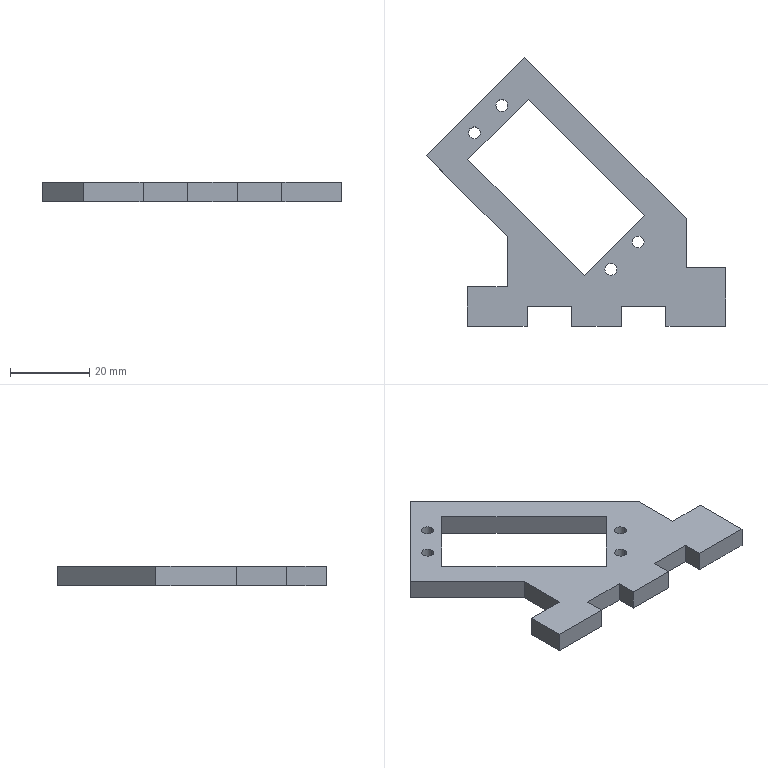Part | SolidWorks | features Extrusion 1 | 1 solid | 32 faces | box 75.329 x 67.7 x 5 mm | volume 9212 mm3 | plane 24 | cylinder 8 | commonest cylinder face diameters 3 x8
STEP:
#1=CARTESIAN_POINT('',(9.961,-20.341,5.));
#2=VERTEX_POINT('',#1);
#3=CARTESIAN_POINT('',(6.961,-20.341,5.));
#4=VERTEX_POINT('',#3);
#5=CARTESIAN_POINT('',(8.461,-20.341,5.));
#6=DIRECTION('',(0.,0.,-1.));
#7=DIRECTION('',(1.,0.,0.));
#8=AXIS2_PLACEMENT_3D('',#5,#6,#7);
#9=CIRCLE('',#8,1.5);
#10=EDGE_CURVE('',#2,#4,#9,.T.);
#11=ORIENTED_EDGE('',*,*,#10,.F.);
#12=CARTESIAN_POINT('',(9.961,-20.341,0.));
#13=VERTEX_POINT('',#12);
#14=CARTESIAN_POINT('',(9.961,-20.341,5.));
#15=DIRECTION('',(0.,0.,-1.));
#16=VECTOR('',#15,1000.);
#17=LINE('',#14,#16);
#18=EDGE_CURVE('',#2,#13,#17,.T.);
#19=ORIENTED_EDGE('',*,*,#18,.T.);
#20=CARTESIAN_POINT('',(6.961,-20.341,0.));
#21=VERTEX_POINT('',#20);
#22=CARTESIAN_POINT('',(8.461,-20.341,0.));
#23=DIRECTION('',(0.,0.,-1.));
#24=DIRECTION('',(1.,0.,0.));
#25=AXIS2_PLACEMENT_3D('',#22,#23,#24);
#26=CIRCLE('',#25,1.5);
#27=EDGE_CURVE('',#13,#21,#26,.T.);
#28=ORIENTED_EDGE('',*,*,#27,.T.);
#29=CARTESIAN_POINT('',(6.961,-20.341,5.));
#30=DIRECTION('',(0.,0.,-1.));
#31=VECTOR('',#30,1000.);
#32=LINE('',#29,#31);
#33=EDGE_CURVE('',#4,#21,#32,.T.);
#34=ORIENTED_EDGE('',*,*,#33,.F.);
#35=EDGE_LOOP('',(#11,#19,#28,#34));
#36=FACE_OUTER_BOUND('',#35,.T.);
#37=CARTESIAN_POINT('',(8.461,-20.341,5.));
#38=DIRECTION('',(0.,0.,-1.));
#39=DIRECTION('',(-1.,0.,0.));
#40=AXIS2_PLACEMENT_3D('',#37,#38,#39);
#41=CYLINDRICAL_SURFACE('',#40,1.5);
#42=ADVANCED_FACE('',(#36),#41,.F.);
#43=CARTESIAN_POINT('',(-20.51,20.918,5.));
#44=VERTEX_POINT('',#43);
#45=CARTESIAN_POINT('',(-17.51,20.918,5.));
#46=VERTEX_POINT('',#45);
#47=CARTESIAN_POINT('',(-19.01,20.918,5.));
#48=DIRECTION('',(0.,0.,1.));
#49=DIRECTION('',(1.,0.,0.));
#50=AXIS2_PLACEMENT_3D('',#47,#48,#49);
#51=CIRCLE('',#50,1.5);
#52=EDGE_CURVE('',#44,#46,#51,.T.);
#53=ORIENTED_EDGE('',*,*,#52,.T.);
#54=CARTESIAN_POINT('',(-17.51,20.918,0.));
#55=VERTEX_POINT('',#54);
#56=CARTESIAN_POINT('',(-17.51,20.918,5.));
#57=DIRECTION('',(0.,0.,-1.));
#58=VECTOR('',#57,1000.);
#59=LINE('',#56,#58);
#60=EDGE_CURVE('',#46,#55,#59,.T.);
#61=ORIENTED_EDGE('',*,*,#60,.T.);
#62=CARTESIAN_POINT('',(-20.51,20.918,0.));
#63=VERTEX_POINT('',#62);
#64=CARTESIAN_POINT('',(-19.01,20.918,0.));
#65=DIRECTION('',(0.,0.,1.));
#66=DIRECTION('',(1.,0.,0.));
#67=AXIS2_PLACEMENT_3D('',#64,#65,#66);
#68=CIRCLE('',#67,1.5);
#69=EDGE_CURVE('',#63,#55,#68,.T.);
#70=ORIENTED_EDGE('',*,*,#69,.F.);
#71=CARTESIAN_POINT('',(-20.51,20.918,5.));
#72=DIRECTION('',(0.,0.,-1.));
#73=VECTOR('',#72,1000.);
#74=LINE('',#71,#73);
#75=EDGE_CURVE('',#44,#63,#74,.T.);
#76=ORIENTED_EDGE('',*,*,#75,.F.);
#77=EDGE_LOOP('',(#53,#61,#70,#76));
#78=FACE_OUTER_BOUND('',#77,.T.);
#79=CARTESIAN_POINT('',(-19.01,20.918,5.));
#80=DIRECTION('',(0.,0.,-1.));
#81=DIRECTION('',(-1.,0.,0.));
#82=AXIS2_PLACEMENT_3D('',#79,#80,#81);
#83=CYLINDRICAL_SURFACE('',#82,1.5);
#84=ADVANCED_FACE('',(#78),#83,.F.);
#85=CARTESIAN_POINT('',(16.856,-13.447,5.));
#86=VERTEX_POINT('',#85);
#87=CARTESIAN_POINT('',(13.856,-13.447,5.));
#88=VERTEX_POINT('',#87);
#89=CARTESIAN_POINT('',(15.356,-13.447,5.));
#90=DIRECTION('',(0.,0.,-1.));
#91=DIRECTION('',(1.,0.,0.));
#92=AXIS2_PLACEMENT_3D('',#89,#90,#91);
#93=CIRCLE('',#92,1.5);
#94=EDGE_CURVE('',#86,#88,#93,.T.);
#95=ORIENTED_EDGE('',*,*,#94,.F.);
#96=CARTESIAN_POINT('',(16.856,-13.447,0.));
#97=VERTEX_POINT('',#96);
#98=CARTESIAN_POINT('',(16.856,-13.447,5.));
#99=DIRECTION('',(0.,0.,-1.));
#100=VECTOR('',#99,1000.);
#101=LINE('',#98,#100);
#102=EDGE_CURVE('',#86,#97,#101,.T.);
#103=ORIENTED_EDGE('',*,*,#102,.T.);
#104=CARTESIAN_POINT('',(13.856,-13.447,0.));
#105=VERTEX_POINT('',#104);
#106=CARTESIAN_POINT('',(15.356,-13.447,0.));
#107=DIRECTION('',(0.,0.,-1.));
#108=DIRECTION('',(1.,0.,0.));
#109=AXIS2_PLACEMENT_3D('',#106,#107,#108);
#110=CIRCLE('',#109,1.5);
#111=EDGE_CURVE('',#97,#105,#110,.T.);
#112=ORIENTED_EDGE('',*,*,#111,.T.);
#113=CARTESIAN_POINT('',(13.856,-13.447,5.));
#114=DIRECTION('',(0.,0.,-1.));
#115=VECTOR('',#114,1000.);
#116=LINE('',#113,#115);
#117=EDGE_CURVE('',#88,#105,#116,.T.);
#118=ORIENTED_EDGE('',*,*,#117,.F.);
#119=EDGE_LOOP('',(#95,#103,#112,#118));
#120=FACE_OUTER_BOUND('',#119,.T.);
#121=CARTESIAN_POINT('',(15.356,-13.447,5.));
#122=DIRECTION('',(0.,0.,-1.));
#123=DIRECTION('',(-1.,0.,0.));
#124=AXIS2_PLACEMENT_3D('',#121,#122,#123);
#125=CYLINDRICAL_SURFACE('',#124,1.5);
#126=ADVANCED_FACE('',(#120),#125,.F.);
#127=CARTESIAN_POINT('',(-27.404,14.024,5.));
#128=VERTEX_POINT('',#127);
#129=CARTESIAN_POINT('',(-24.404,14.024,5.));
#130=VERTEX_POINT('',#129);
#131=CARTESIAN_POINT('',(-25.904,14.024,5.));
#132=DIRECTION('',(0.,0.,1.));
#133=DIRECTION('',(1.,0.,0.));
#134=AXIS2_PLACEMENT_3D('',#131,#132,#133);
#135=CIRCLE('',#134,1.5);
#136=EDGE_CURVE('',#128,#130,#135,.T.);
#137=ORIENTED_EDGE('',*,*,#136,.T.);
#138=CARTESIAN_POINT('',(-24.404,14.024,0.));
#139=VERTEX_POINT('',#138);
#140=CARTESIAN_POINT('',(-24.404,14.024,5.));
#141=DIRECTION('',(0.,0.,-1.));
#142=VECTOR('',#141,1000.);
#143=LINE('',#140,#142);
#144=EDGE_CURVE('',#130,#139,#143,.T.);
#145=ORIENTED_EDGE('',*,*,#144,.T.);
#146=CARTESIAN_POINT('',(-27.404,14.024,0.));
#147=VERTEX_POINT('',#146);
#148=CARTESIAN_POINT('',(-25.904,14.024,0.));
#149=DIRECTION('',(0.,0.,1.));
#150=DIRECTION('',(1.,0.,0.));
#151=AXIS2_PLACEMENT_3D('',#148,#149,#150);
#152=CIRCLE('',#151,1.5);
#153=EDGE_CURVE('',#147,#139,#152,.T.);
#154=ORIENTED_EDGE('',*,*,#153,.F.);
#155=CARTESIAN_POINT('',(-27.404,14.024,5.));
#156=DIRECTION('',(0.,0.,-1.));
#157=VECTOR('',#156,1000.);
#158=LINE('',#155,#157);
#159=EDGE_CURVE('',#128,#147,#158,.T.);
#160=ORIENTED_EDGE('',*,*,#159,.F.);
#161=EDGE_LOOP('',(#137,#145,#154,#160));
#162=FACE_OUTER_BOUND('',#161,.T.);
#163=CARTESIAN_POINT('',(-25.904,14.024,5.));
#164=DIRECTION('',(0.,0.,-1.));
#165=DIRECTION('',(-1.,0.,0.));
#166=AXIS2_PLACEMENT_3D('',#163,#164,#165);
#167=CYLINDRICAL_SURFACE('',#166,1.5);
#168=ADVANCED_FACE('',(#162),#167,.F.);
#169=CARTESIAN_POINT('',(-12.649,-29.708,0.));
#170=VERTEX_POINT('',#169);
#171=CARTESIAN_POINT('',(-12.649,-34.708,0.));
#172=VERTEX_POINT('',#171);
#173=CARTESIAN_POINT('',(-12.649,0.,0.));
#174=DIRECTION('',(0.,-1.,0.));
#175=VECTOR('',#174,1000.);
#176=LINE('',#173,#175);
#177=EDGE_CURVE('',#170,#172,#176,.T.);
#178=ORIENTED_EDGE('',*,*,#177,.F.);
#179=CARTESIAN_POINT('',(-12.649,-29.708,5.));
#180=VERTEX_POINT('',#179);
#181=CARTESIAN_POINT('',(-12.649,-29.708,5.));
#182=DIRECTION('',(0.,0.,-1.));
#183=VECTOR('',#182,1000.);
#184=LINE('',#181,#183);
#185=EDGE_CURVE('',#180,#170,#184,.T.);
#186=ORIENTED_EDGE('',*,*,#185,.F.);
#187=CARTESIAN_POINT('',(-12.649,-34.708,5.));
#188=VERTEX_POINT('',#187);
#189=CARTESIAN_POINT('',(-12.649,0.,5.));
#190=DIRECTION('',(0.,-1.,0.));
#191=VECTOR('',#190,1000.);
#192=LINE('',#189,#191);
#193=EDGE_CURVE('',#180,#188,#192,.T.);
#194=ORIENTED_EDGE('',*,*,#193,.T.);
#195=CARTESIAN_POINT('',(-12.649,-34.708,5.));
#196=DIRECTION('',(0.,0.,-1.));
#197=VECTOR('',#196,1000.);
#198=LINE('',#195,#197);
#199=EDGE_CURVE('',#188,#172,#198,.T.);
#200=ORIENTED_EDGE('',*,*,#199,.T.);
#201=EDGE_LOOP('',(#178,#186,#194,#200));
#202=FACE_OUTER_BOUND('',#201,.T.);
#203=CARTESIAN_POINT('',(-12.649,0.,5.));
#204=DIRECTION('',(1.,0.,0.));
#205=DIRECTION('',(0.,0.,-1.));
#206=AXIS2_PLACEMENT_3D('',#203,#204,#205);
#207=PLANE('',#206);
#208=ADVANCED_FACE('',(#202),#207,.T.);
#209=CARTESIAN_POINT('',(-1.399,-29.708,0.));
#210=VERTEX_POINT('',#209);
#211=CARTESIAN_POINT('',(0.,-29.708,0.));
#212=DIRECTION('',(-1.,0.,0.));
#213=VECTOR('',#212,1000.);
#214=LINE('',#211,#213);
#215=EDGE_CURVE('',#210,#170,#214,.T.);
#216=ORIENTED_EDGE('',*,*,#215,.F.);
#217=CARTESIAN_POINT('',(-1.399,-29.708,5.));
#218=VERTEX_POINT('',#217);
#219=CARTESIAN_POINT('',(-1.399,-29.708,5.));
#220=DIRECTION('',(0.,0.,-1.));
#221=VECTOR('',#220,1000.);
#222=LINE('',#219,#221);
#223=EDGE_CURVE('',#218,#210,#222,.T.);
#224=ORIENTED_EDGE('',*,*,#223,.F.);
#225=CARTESIAN_POINT('',(0.,-29.708,5.));
#226=DIRECTION('',(-1.,0.,0.));
#227=VECTOR('',#226,1000.);
#228=LINE('',#225,#227);
#229=EDGE_CURVE('',#218,#180,#228,.T.);
#230=ORIENTED_EDGE('',*,*,#229,.T.);
#231=ORIENTED_EDGE('',*,*,#185,.T.);
#232=EDGE_LOOP('',(#216,#224,#230,#231));
#233=FACE_OUTER_BOUND('',#232,.T.);
#234=CARTESIAN_POINT('',(0.,-29.708,5.));
#235=DIRECTION('',(0.,-1.,0.));
#236=DIRECTION('',(0.,0.,-1.));
#237=AXIS2_PLACEMENT_3D('',#234,#235,#236);
#238=PLANE('',#237);
#239=ADVANCED_FACE('',(#233),#238,.T.);
#240=CARTESIAN_POINT('',(-1.399,-34.708,0.));
#241=VERTEX_POINT('',#240);
#242=CARTESIAN_POINT('',(-1.399,0.,0.));
#243=DIRECTION('',(0.,1.,0.));
#244=VECTOR('',#243,1000.);
#245=LINE('',#242,#244);
#246=EDGE_CURVE('',#241,#210,#245,.T.);
#247=ORIENTED_EDGE('',*,*,#246,.F.);
#248=CARTESIAN_POINT('',(-1.399,-34.708,5.));
#249=VERTEX_POINT('',#248);
#250=CARTESIAN_POINT('',(-1.399,-34.708,5.));
#251=DIRECTION('',(0.,0.,-1.));
#252=VECTOR('',#251,1000.);
#253=LINE('',#250,#252);
#254=EDGE_CURVE('',#249,#241,#253,.T.);
#255=ORIENTED_EDGE('',*,*,#254,.F.);
#256=CARTESIAN_POINT('',(-1.399,0.,5.));
#257=DIRECTION('',(0.,1.,0.));
#258=VECTOR('',#257,1000.);
#259=LINE('',#256,#258);
#260=EDGE_CURVE('',#249,#218,#259,.T.);
#261=ORIENTED_EDGE('',*,*,#260,.T.);
#262=ORIENTED_EDGE('',*,*,#223,.T.);
#263=EDGE_LOOP('',(#247,#255,#261,#262));
#264=FACE_OUTER_BOUND('',#263,.T.);
#265=CARTESIAN_POINT('',(-1.399,0.,5.));
#266=DIRECTION('',(-1.,0.,0.));
#267=DIRECTION('',(0.,-1.,0.));
#268=AXIS2_PLACEMENT_3D('',#265,#266,#267);
#269=PLANE('',#268);
#270=ADVANCED_FACE('',(#264),#269,.T.);
#271=CARTESIAN_POINT('',(11.101,-34.708,0.));
#272=VERTEX_POINT('',#271);
#273=CARTESIAN_POINT('',(0.,-34.708,0.));
#274=DIRECTION('',(-1.,0.,0.));
#275=VECTOR('',#274,1000.);
#276=LINE('',#273,#275);
#277=EDGE_CURVE('',#272,#241,#276,.T.);
#278=ORIENTED_EDGE('',*,*,#277,.F.);
#279=CARTESIAN_POINT('',(11.101,-34.708,5.));
#280=VERTEX_POINT('',#279);
#281=CARTESIAN_POINT('',(11.101,-34.708,5.));
#282=DIRECTION('',(0.,0.,-1.));
#283=VECTOR('',#282,1000.);
#284=LINE('',#281,#283);
#285=EDGE_CURVE('',#280,#272,#284,.T.);
#286=ORIENTED_EDGE('',*,*,#285,.F.);
#287=CARTESIAN_POINT('',(0.,-34.708,5.));
#288=DIRECTION('',(-1.,0.,0.));
#289=VECTOR('',#288,1000.);
#290=LINE('',#287,#289);
#291=EDGE_CURVE('',#280,#249,#290,.T.);
#292=ORIENTED_EDGE('',*,*,#291,.T.);
#293=ORIENTED_EDGE('',*,*,#254,.T.);
#294=EDGE_LOOP('',(#278,#286,#292,#293));
#295=FACE_OUTER_BOUND('',#294,.T.);
#296=CARTESIAN_POINT('',(0.,-34.708,5.));
#297=DIRECTION('',(0.,-1.,0.));
#298=DIRECTION('',(1.,0.,0.));
#299=AXIS2_PLACEMENT_3D('',#296,#297,#298);
#300=PLANE('',#299);
#301=ADVANCED_FACE('',(#295),#300,.T.);
#302=CARTESIAN_POINT('',(11.101,-29.708,0.));
#303=VERTEX_POINT('',#302);
#304=CARTESIAN_POINT('',(11.101,0.,0.));
#305=DIRECTION('',(0.,-1.,0.));
#306=VECTOR('',#305,1000.);
#307=LINE('',#304,#306);
#308=EDGE_CURVE('',#303,#272,#307,.T.);
#309=ORIENTED_EDGE('',*,*,#308,.F.);
#310=CARTESIAN_POINT('',(11.101,-29.708,5.));
#311=VERTEX_POINT('',#310);
#312=CARTESIAN_POINT('',(11.101,-29.708,5.));
#313=DIRECTION('',(0.,0.,-1.));
#314=VECTOR('',#313,1000.);
#315=LINE('',#312,#314);
#316=EDGE_CURVE('',#311,#303,#315,.T.);
#317=ORIENTED_EDGE('',*,*,#316,.F.);
#318=CARTESIAN_POINT('',(11.101,0.,5.));
#319=DIRECTION('',(0.,-1.,0.));
#320=VECTOR('',#319,1000.);
#321=LINE('',#318,#320);
#322=EDGE_CURVE('',#311,#280,#321,.T.);
#323=ORIENTED_EDGE('',*,*,#322,.T.);
#324=ORIENTED_EDGE('',*,*,#285,.T.);
#325=EDGE_LOOP('',(#309,#317,#323,#324));
#326=FACE_OUTER_BOUND('',#325,.T.);
#327=CARTESIAN_POINT('',(11.101,0.,5.));
#328=DIRECTION('',(1.,0.,0.));
#329=DIRECTION('',(0.,0.,-1.));
#330=AXIS2_PLACEMENT_3D('',#327,#328,#329);
#331=PLANE('',#330);
#332=ADVANCED_FACE('',(#326),#331,.T.);
#333=CARTESIAN_POINT('',(22.351,-29.708,0.));
#334=VERTEX_POINT('',#333);
#335=CARTESIAN_POINT('',(0.,-29.708,0.));
#336=DIRECTION('',(-1.,0.,0.));
#337=VECTOR('',#336,1000.);
#338=LINE('',#335,#337);
#339=EDGE_CURVE('',#334,#303,#338,.T.);
#340=ORIENTED_EDGE('',*,*,#339,.F.);
#341=CARTESIAN_POINT('',(22.351,-29.708,5.));
#342=VERTEX_POINT('',#341);
#343=CARTESIAN_POINT('',(22.351,-29.708,5.));
#344=DIRECTION('',(0.,0.,-1.));
#345=VECTOR('',#344,1000.);
#346=LINE('',#343,#345);
#347=EDGE_CURVE('',#342,#334,#346,.T.);
#348=ORIENTED_EDGE('',*,*,#347,.F.);
#349=CARTESIAN_POINT('',(0.,-29.708,5.));
#350=DIRECTION('',(-1.,0.,0.));
#351=VECTOR('',#350,1000.);
#352=LINE('',#349,#351);
#353=EDGE_CURVE('',#342,#311,#352,.T.);
#354=ORIENTED_EDGE('',*,*,#353,.T.);
#355=ORIENTED_EDGE('',*,*,#316,.T.);
#356=EDGE_LOOP('',(#340,#348,#354,#355));
#357=FACE_OUTER_BOUND('',#356,.T.);
#358=CARTESIAN_POINT('',(0.,-29.708,5.));
#359=DIRECTION('',(0.,-1.,0.));
#360=DIRECTION('',(0.,0.,-1.));
#361=AXIS2_PLACEMENT_3D('',#358,#359,#360);
#362=PLANE('',#361);
#363=ADVANCED_FACE('',(#357),#362,.T.);
#364=CARTESIAN_POINT('',(22.351,-34.708,0.));
#365=VERTEX_POINT('',#364);
#366=CARTESIAN_POINT('',(22.351,0.,0.));
#367=DIRECTION('',(0.,1.,0.));
#368=VECTOR('',#367,1000.);
#369=LINE('',#366,#368);
#370=EDGE_CURVE('',#365,#334,#369,.T.);
#371=ORIENTED_EDGE('',*,*,#370,.F.);
#372=CARTESIAN_POINT('',(22.351,-34.708,5.));
#373=VERTEX_POINT('',#372);
#374=CARTESIAN_POINT('',(22.351,-34.708,5.));
#375=DIRECTION('',(0.,0.,-1.));
#376=VECTOR('',#375,1000.);
#377=LINE('',#374,#376);
#378=EDGE_CURVE('',#373,#365,#377,.T.);
#379=ORIENTED_EDGE('',*,*,#378,.F.);
#380=CARTESIAN_POINT('',(22.351,0.,5.));
#381=DIRECTION('',(0.,1.,0.));
#382=VECTOR('',#381,1000.);
#383=LINE('',#380,#382);
#384=EDGE_CURVE('',#373,#342,#383,.T.);
#385=ORIENTED_EDGE('',*,*,#384,.T.);
#386=ORIENTED_EDGE('',*,*,#347,.T.);
#387=EDGE_LOOP('',(#371,#379,#385,#386));
#388=FACE_OUTER_BOUND('',#387,.T.);
#389=CARTESIAN_POINT('',(22.351,0.,5.));
#390=DIRECTION('',(-1.,0.,0.));
#391=DIRECTION('',(0.,0.,1.));
#392=AXIS2_PLACEMENT_3D('',#389,#390,#391);
#393=PLANE('',#392);
#394=ADVANCED_FACE('',(#388),#393,.T.);
#395=CARTESIAN_POINT('',(37.351,-34.708,0.));
#396=VERTEX_POINT('',#395);
#397=CARTESIAN_POINT('',(0.,-34.708,0.));
#398=DIRECTION('',(-1.,0.,0.));
#399=VECTOR('',#398,1000.);
#400=LINE('',#397,#399);
#401=EDGE_CURVE('',#396,#365,#400,.T.);
#402=ORIENTED_EDGE('',*,*,#401,.F.);
#403=CARTESIAN_POINT('',(37.351,-34.708,5.));
#404=VERTEX_POINT('',#403);
#405=CARTESIAN_POINT('',(37.351,-34.708,5.));
#406=DIRECTION('',(0.,0.,-1.));
#407=VECTOR('',#406,1000.);
#408=LINE('',#405,#407);
#409=EDGE_CURVE('',#404,#396,#408,.T.);
#410=ORIENTED_EDGE('',*,*,#409,.F.);
#411=CARTESIAN_POINT('',(0.,-34.708,5.));
#412=DIRECTION('',(-1.,0.,0.));
#413=VECTOR('',#412,1000.);
#414=LINE('',#411,#413);
#415=EDGE_CURVE('',#404,#373,#414,.T.);
#416=ORIENTED_EDGE('',*,*,#415,.T.);
#417=ORIENTED_EDGE('',*,*,#378,.T.);
#418=EDGE_LOOP('',(#402,#410,#416,#417));
#419=FACE_OUTER_BOUND('',#418,.T.);
#420=CARTESIAN_POINT('',(0.,-34.708,5.));
#421=DIRECTION('',(0.,-1.,0.));
#422=DIRECTION('',(0.,0.,-1.));
#423=AXIS2_PLACEMENT_3D('',#420,#421,#422);
#424=PLANE('',#423);
#425=ADVANCED_FACE('',(#419),#424,.T.);
#426=CARTESIAN_POINT('',(37.351,-19.908,0.));
#427=VERTEX_POINT('',#426);
#428=CARTESIAN_POINT('',(37.351,0.,0.));
#429=DIRECTION('',(0.,-1.,0.));
#430=VECTOR('',#429,1000.);
#431=LINE('',#428,#430);
#432=EDGE_CURVE('',#427,#396,#431,.T.);
#433=ORIENTED_EDGE('',*,*,#432,.F.);
#434=CARTESIAN_POINT('',(37.351,-19.908,5.));
#435=VERTEX_POINT('',#434);
#436=CARTESIAN_POINT('',(37.351,-19.908,5.));
#437=DIRECTION('',(0.,0.,-1.));
#438=VECTOR('',#437,1000.);
#439=LINE('',#436,#438);
#440=EDGE_CURVE('',#435,#427,#439,.T.);
#441=ORIENTED_EDGE('',*,*,#440,.F.);
#442=CARTESIAN_POINT('',(37.351,0.,5.));
#443=DIRECTION('',(0.,-1.,0.));
#444=VECTOR('',#443,1000.);
#445=LINE('',#442,#444);
#446=EDGE_CURVE('',#435,#404,#445,.T.);
#447=ORIENTED_EDGE('',*,*,#446,.T.);
#448=ORIENTED_EDGE('',*,*,#409,.T.);
#449=EDGE_LOOP('',(#433,#441,#447,#448));
#450=FACE_OUTER_BOUND('',#449,.T.);
#451=CARTESIAN_POINT('',(37.351,0.,5.));
#452=DIRECTION('',(1.,0.,0.));
#453=DIRECTION('',(0.,1.,0.));
#454=AXIS2_PLACEMENT_3D('',#451,#452,#453);
#455=PLANE('',#454);
#456=ADVANCED_FACE('',(#450),#455,.T.);
#457=CARTESIAN_POINT('',(27.421,-19.908,0.));
#458=VERTEX_POINT('',#457);
#459=CARTESIAN_POINT('',(0.,-19.908,0.));
#460=DIRECTION('',(1.,0.,0.));
#461=VECTOR('',#460,1000.);
#462=LINE('',#459,#461);
#463=EDGE_CURVE('',#458,#427,#462,.T.);
#464=ORIENTED_EDGE('',*,*,#463,.F.);
#465=CARTESIAN_POINT('',(27.421,-19.908,5.));
#466=VERTEX_POINT('',#465);
#467=CARTESIAN_POINT('',(27.421,-19.908,5.));
#468=DIRECTION('',(0.,0.,-1.));
#469=VECTOR('',#468,1000.);
#470=LINE('',#467,#469);
#471=EDGE_CURVE('',#466,#458,#470,.T.);
#472=ORIENTED_EDGE('',*,*,#471,.F.);
#473=CARTESIAN_POINT('',(0.,-19.908,5.));
#474=DIRECTION('',(1.,0.,0.));
#475=VECTOR('',#474,1000.);
#476=LINE('',#473,#475);
#477=EDGE_CURVE('',#466,#435,#476,.T.);
#478=ORIENTED_EDGE('',*,*,#477,.T.);
#479=ORIENTED_EDGE('',*,*,#440,.T.);
#480=EDGE_LOOP('',(#464,#472,#478,#479));
#481=FACE_OUTER_BOUND('',#480,.T.);
#482=CARTESIAN_POINT('',(0.,-19.908,5.));
#483=DIRECTION('',(0.,1.,0.));
#484=DIRECTION('',(-1.,0.,0.));
#485=AXIS2_PLACEMENT_3D('',#482,#483,#484);
#486=PLANE('',#485);
#487=ADVANCED_FACE('',(#481),#486,.T.);
#488=CARTESIAN_POINT('',(27.421,-7.658,0.));
#489=VERTEX_POINT('',#488);
#490=CARTESIAN_POINT('',(27.421,0.,0.));
#491=DIRECTION('',(0.,-1.,0.));
#492=VECTOR('',#491,1000.);
#493=LINE('',#490,#492);
#494=EDGE_CURVE('',#489,#458,#493,.T.);
#495=ORIENTED_EDGE('',*,*,#494,.F.);
#496=CARTESIAN_POINT('',(27.421,-7.658,5.));
#497=VERTEX_POINT('',#496);
#498=CARTESIAN_POINT('',(27.421,-7.658,5.));
#499=DIRECTION('',(0.,0.,-1.));
#500=VECTOR('',#499,1000.);
#501=LINE('',#498,#500);
#502=EDGE_CURVE('',#497,#489,#501,.T.);
#503=ORIENTED_EDGE('',*,*,#502,.F.);
#504=CARTESIAN_POINT('',(27.421,0.,5.));
#505=DIRECTION('',(0.,-1.,0.));
#506=VECTOR('',#505,1000.);
#507=LINE('',#504,#506);
#508=EDGE_CURVE('',#497,#466,#507,.T.);
#509=ORIENTED_EDGE('',*,*,#508,.T.);
#510=ORIENTED_EDGE('',*,*,#471,.T.);
#511=EDGE_LOOP('',(#495,#503,#509,#510));
#512=FACE_OUTER_BOUND('',#511,.T.);
#513=CARTESIAN_POINT('',(27.421,0.,5.));
#514=DIRECTION('',(1.,0.,0.));
#515=DIRECTION('',(0.,1.,0.));
#516=AXIS2_PLACEMENT_3D('',#513,#514,#515);
#517=PLANE('',#516);
#518=ADVANCED_FACE('',(#512),#517,.T.);
#519=CARTESIAN_POINT('',(-13.229,32.992,0.));
#520=VERTEX_POINT('',#519);
#521=CARTESIAN_POINT('',(9.882,9.882,0.));
#522=DIRECTION('',(0.7071,-0.7071,0.));
#523=VECTOR('',#522,1000.);
#524=LINE('',#521,#523);
#525=EDGE_CURVE('',#520,#489,#524,.T.);
#526=ORIENTED_EDGE('',*,*,#525,.F.);
#527=CARTESIAN_POINT('',(-13.229,32.992,5.));
#528=VERTEX_POINT('',#527);
#529=CARTESIAN_POINT('',(-13.229,32.992,5.));
#530=DIRECTION('',(0.,0.,-1.));
#531=VECTOR('',#530,1000.);
#532=LINE('',#529,#531);
#533=EDGE_CURVE('',#528,#520,#532,.T.);
#534=ORIENTED_EDGE('',*,*,#533,.F.);
#535=CARTESIAN_POINT('',(9.882,9.882,5.));
#536=DIRECTION('',(0.7071,-0.7071,0.));
#537=VECTOR('',#536,1000.);
#538=LINE('',#535,#537);
#539=EDGE_CURVE('',#528,#497,#538,.T.);
#540=ORIENTED_EDGE('',*,*,#539,.T.);
#541=ORIENTED_EDGE('',*,*,#502,.T.);
#542=EDGE_LOOP('',(#526,#534,#540,#541));
#543=FACE_OUTER_BOUND('',#542,.T.);
#544=CARTESIAN_POINT('',(9.882,9.882,5.));
#545=DIRECTION('',(0.7071,0.7071,0.));
#546=DIRECTION('',(-0.7071,0.7071,0.));
#547=AXIS2_PLACEMENT_3D('',#544,#545,#546);
#548=PLANE('',#547);
#549=ADVANCED_FACE('',(#543),#548,.T.);
#550=CARTESIAN_POINT('',(-37.978,8.243,0.));
#551=VERTEX_POINT('',#550);
#552=CARTESIAN_POINT('',(-23.111,23.111,0.));
#553=DIRECTION('',(0.7071,0.7071,0.));
#554=VECTOR('',#553,1000.);
#555=LINE('',#552,#554);
#556=EDGE_CURVE('',#551,#520,#555,.T.);
#557=ORIENTED_EDGE('',*,*,#556,.F.);
#558=CARTESIAN_POINT('',(-37.978,8.243,5.));
#559=VERTEX_POINT('',#558);
#560=CARTESIAN_POINT('',(-37.978,8.243,5.));
#561=DIRECTION('',(0.,0.,-1.));
#562=VECTOR('',#561,1000.);
#563=LINE('',#560,#562);
#564=EDGE_CURVE('',#559,#551,#563,.T.);
#565=ORIENTED_EDGE('',*,*,#564,.F.);
#566=CARTESIAN_POINT('',(-23.111,23.111,5.));
#567=DIRECTION('',(0.7071,0.7071,0.));
#568=VECTOR('',#567,1000.);
#569=LINE('',#566,#568);
#570=EDGE_CURVE('',#559,#528,#569,.T.);
#571=ORIENTED_EDGE('',*,*,#570,.T.);
#572=ORIENTED_EDGE('',*,*,#533,.T.);
#573=EDGE_LOOP('',(#557,#565,#571,#572));
#574=FACE_OUTER_BOUND('',#573,.T.);
#575=CARTESIAN_POINT('',(-23.111,23.111,5.));
#576=DIRECTION('',(-0.7071,0.7071,0.));
#577=DIRECTION('',(-0.7071,-0.7071,0.));
#578=AXIS2_PLACEMENT_3D('',#575,#576,#577);
#579=PLANE('',#578);
#580=ADVANCED_FACE('',(#574),#579,.T.);
#581=CARTESIAN_POINT('',(-17.649,-12.086,0.));
#582=VERTEX_POINT('',#581);
#583=CARTESIAN_POINT('',(-14.867,-14.867,0.));
#584=DIRECTION('',(-0.7071,0.7071,0.));
#585=VECTOR('',#584,1000.);
#586=LINE('',#583,#585);
#587=EDGE_CURVE('',#582,#551,#586,.T.);
#588=ORIENTED_EDGE('',*,*,#587,.F.);
#589=CARTESIAN_POINT('',(-17.649,-12.086,5.));
#590=VERTEX_POINT('',#589);
#591=CARTESIAN_POINT('',(-17.649,-12.086,5.));
#592=DIRECTION('',(0.,0.,-1.));
#593=VECTOR('',#592,1000.);
#594=LINE('',#591,#593);
#595=EDGE_CURVE('',#590,#582,#594,.T.);
#596=ORIENTED_EDGE('',*,*,#595,.F.);
#597=CARTESIAN_POINT('',(-14.867,-14.867,5.));
#598=DIRECTION('',(-0.7071,0.7071,0.));
#599=VECTOR('',#598,1000.);
#600=LINE('',#597,#599);
#601=EDGE_CURVE('',#590,#559,#600,.T.);
#602=ORIENTED_EDGE('',*,*,#601,.T.);
#603=ORIENTED_EDGE('',*,*,#564,.T.);
#604=EDGE_LOOP('',(#588,#596,#602,#603));
#605=FACE_OUTER_BOUND('',#604,.T.);
#606=CARTESIAN_POINT('',(-14.867,-14.867,5.));
#607=DIRECTION('',(-0.7071,-0.7071,0.));
#608=DIRECTION('',(0.7071,-0.7071,0.));
#609=AXIS2_PLACEMENT_3D('',#606,#607,#608);
#610=PLANE('',#609);
#611=ADVANCED_FACE('',(#605),#610,.T.);
#612=CARTESIAN_POINT('',(-17.649,-24.708,0.));
#613=VERTEX_POINT('',#612);
#614=CARTESIAN_POINT('',(-17.649,0.,0.));
#615=DIRECTION('',(0.,1.,0.));
#616=VECTOR('',#615,1000.);
#617=LINE('',#614,#616);
#618=EDGE_CURVE('',#613,#582,#617,.T.);
#619=ORIENTED_EDGE('',*,*,#618,.F.);
#620=CARTESIAN_POINT('',(-17.649,-24.708,5.));
#621=VERTEX_POINT('',#620);
#622=CARTESIAN_POINT('',(-17.649,-24.708,5.));
#623=DIRECTION('',(0.,0.,-1.));
#624=VECTOR('',#623,1000.);
#625=LINE('',#622,#624);
#626=EDGE_CURVE('',#621,#613,#625,.T.);
#627=ORIENTED_EDGE('',*,*,#626,.F.);
#628=CARTESIAN_POINT('',(-17.649,0.,5.));
#629=DIRECTION('',(0.,1.,0.));
#630=VECTOR('',#629,1000.);
#631=LINE('',#628,#630);
#632=EDGE_CURVE('',#621,#590,#631,.T.);
#633=ORIENTED_EDGE('',*,*,#632,.T.);
#634=ORIENTED_EDGE('',*,*,#595,.T.);
#635=EDGE_LOOP('',(#619,#627,#633,#634));
#636=FACE_OUTER_BOUND('',#635,.T.);
#637=CARTESIAN_POINT('',(-17.649,0.,5.));
#638=DIRECTION('',(-1.,0.,0.));
#639=DIRECTION('',(0.,-1.,0.));
#640=AXIS2_PLACEMENT_3D('',#637,#638,#639);
#641=PLANE('',#640);
#642=ADVANCED_FACE('',(#636),#641,.T.);
#643=CARTESIAN_POINT('',(-27.649,-24.708,0.));
#644=VERTEX_POINT('',#643);
#645=CARTESIAN_POINT('',(0.,-24.708,0.));
#646=DIRECTION('',(1.,0.,0.));
#647=VECTOR('',#646,1000.);
#648=LINE('',#645,#647);
#649=EDGE_CURVE('',#644,#613,#648,.T.);
#650=ORIENTED_EDGE('',*,*,#649,.F.);
#651=CARTESIAN_POINT('',(-27.649,-24.708,5.));
#652=VERTEX_POINT('',#651);
#653=CARTESIAN_POINT('',(-27.649,-24.708,5.));
#654=DIRECTION('',(0.,0.,-1.));
#655=VECTOR('',#654,1000.);
#656=LINE('',#653,#655);
#657=EDGE_CURVE('',#652,#644,#656,.T.);
#658=ORIENTED_EDGE('',*,*,#657,.F.);
#659=CARTESIAN_POINT('',(0.,-24.708,5.));
#660=DIRECTION('',(1.,0.,0.));
#661=VECTOR('',#660,1000.);
#662=LINE('',#659,#661);
#663=EDGE_CURVE('',#652,#621,#662,.T.);
#664=ORIENTED_EDGE('',*,*,#663,.T.);
#665=ORIENTED_EDGE('',*,*,#626,.T.);
#666=EDGE_LOOP('',(#650,#658,#664,#665));
#667=FACE_OUTER_BOUND('',#666,.T.);
#668=CARTESIAN_POINT('',(0.,-24.708,5.));
#669=DIRECTION('',(0.,1.,0.));
#670=DIRECTION('',(-1.,0.,0.));
#671=AXIS2_PLACEMENT_3D('',#668,#669,#670);
#672=PLANE('',#671);
#673=ADVANCED_FACE('',(#667),#672,.T.);
#674=CARTESIAN_POINT('',(-27.649,-34.708,0.));
#675=VERTEX_POINT('',#674);
#676=CARTESIAN_POINT('',(-27.649,0.,0.));
#677=DIRECTION('',(0.,1.,0.));
#678=VECTOR('',#677,1000.);
#679=LINE('',#676,#678);
#680=EDGE_CURVE('',#675,#644,#679,.T.);
#681=ORIENTED_EDGE('',*,*,#680,.F.);
#682=CARTESIAN_POINT('',(-27.649,-34.708,5.));
#683=VERTEX_POINT('',#682);
#684=CARTESIAN_POINT('',(-27.649,-34.708,5.));
#685=DIRECTION('',(0.,0.,-1.));
#686=VECTOR('',#685,1000.);
#687=LINE('',#684,#686);
#688=EDGE_CURVE('',#683,#675,#687,.T.);
#689=ORIENTED_EDGE('',*,*,#688,.F.);
#690=CARTESIAN_POINT('',(-27.649,0.,5.));
#691=DIRECTION('',(0.,1.,0.));
#692=VECTOR('',#691,1000.);
#693=LINE('',#690,#692);
#694=EDGE_CURVE('',#683,#652,#693,.T.);
#695=ORIENTED_EDGE('',*,*,#694,.T.);
#696=ORIENTED_EDGE('',*,*,#657,.T.);
#697=EDGE_LOOP('',(#681,#689,#695,#696));
#698=FACE_OUTER_BOUND('',#697,.T.);
#699=CARTESIAN_POINT('',(-27.649,0.,5.));
#700=DIRECTION('',(-1.,0.,0.));
#701=DIRECTION('',(0.,-1.,0.));
#702=AXIS2_PLACEMENT_3D('',#699,#700,#701);
#703=PLANE('',#702);
#704=ADVANCED_FACE('',(#698),#703,.T.);
#705=CARTESIAN_POINT('',(-12.345,22.562,0.));
#706=VERTEX_POINT('',#705);
#707=CARTESIAN_POINT('',(-27.548,7.36,0.));
#708=VERTEX_POINT('',#707);
#709=CARTESIAN_POINT('',(-17.454,17.454,0.));
#710=DIRECTION('',(-0.7071,-0.7071,0.));
#711=VECTOR('',#710,1000.);
#712=LINE('',#709,#711);
#713=EDGE_CURVE('',#706,#708,#712,.T.);
#714=ORIENTED_EDGE('',*,*,#713,.F.);
#715=CARTESIAN_POINT('',(-12.345,22.562,5.));
#716=VERTEX_POINT('',#715);
#717=CARTESIAN_POINT('',(-12.345,22.562,5.));
#718=DIRECTION('',(0.,0.,-1.));
#719=VECTOR('',#718,1000.);
#720=LINE('',#717,#719);
#721=EDGE_CURVE('',#716,#706,#720,.T.);
#722=ORIENTED_EDGE('',*,*,#721,.F.);
#723=CARTESIAN_POINT('',(-27.548,7.36,5.));
#724=VERTEX_POINT('',#723);
#725=CARTESIAN_POINT('',(-17.454,17.454,5.));
#726=DIRECTION('',(-0.7071,-0.7071,0.));
#727=VECTOR('',#726,1000.);
#728=LINE('',#725,#727);
#729=EDGE_CURVE('',#716,#724,#728,.T.);
#730=ORIENTED_EDGE('',*,*,#729,.T.);
#731=CARTESIAN_POINT('',(-27.548,7.36,5.));
#732=DIRECTION('',(0.,0.,-1.));
#733=VECTOR('',#732,1000.);
#734=LINE('',#731,#733);
#735=EDGE_CURVE('',#724,#708,#734,.T.);
#736=ORIENTED_EDGE('',*,*,#735,.T.);
#737=EDGE_LOOP('',(#714,#722,#730,#736));
#738=FACE_OUTER_BOUND('',#737,.T.);
#739=CARTESIAN_POINT('',(-17.454,17.454,5.));
#740=DIRECTION('',(0.7071,-0.7071,0.));
#741=DIRECTION('',(0.7071,0.7071,0.));
#742=AXIS2_PLACEMENT_3D('',#739,#740,#741);
#743=PLANE('',#742);
#744=ADVANCED_FACE('',(#738),#743,.T.);
#745=CARTESIAN_POINT('',(17.,-6.783,0.));
#746=VERTEX_POINT('',#745);
#747=CARTESIAN_POINT('',(5.109,5.109,0.));
#748=DIRECTION('',(-0.7071,0.7071,0.));
#749=VECTOR('',#748,1000.);
#750=LINE('',#747,#749);
#751=EDGE_CURVE('',#746,#706,#750,.T.);
#752=ORIENTED_EDGE('',*,*,#751,.F.);
#753=CARTESIAN_POINT('',(17.,-6.783,5.));
#754=VERTEX_POINT('',#753);
#755=CARTESIAN_POINT('',(17.,-6.783,5.));
#756=DIRECTION('',(0.,0.,-1.));
#757=VECTOR('',#756,1000.);
#758=LINE('',#755,#757);
#759=EDGE_CURVE('',#754,#746,#758,.T.);
#760=ORIENTED_EDGE('',*,*,#759,.F.);
#761=CARTESIAN_POINT('',(5.109,5.109,5.));
#762=DIRECTION('',(-0.7071,0.7071,0.));
#763=VECTOR('',#762,1000.);
#764=LINE('',#761,#763);
#765=EDGE_CURVE('',#754,#716,#764,.T.);
#766=ORIENTED_EDGE('',*,*,#765,.T.);
#767=ORIENTED_EDGE('',*,*,#721,.T.);
#768=EDGE_LOOP('',(#752,#760,#766,#767));
#769=FACE_OUTER_BOUND('',#768,.T.);
#770=CARTESIAN_POINT('',(5.109,5.109,5.));
#771=DIRECTION('',(-0.7071,-0.7071,0.));
#772=DIRECTION('',(0.7071,-0.7071,0.));
#773=AXIS2_PLACEMENT_3D('',#770,#771,#772);
#774=PLANE('',#773);
#775=ADVANCED_FACE('',(#769),#774,.T.);
#776=CARTESIAN_POINT('',(1.797,-21.985,0.));
#777=VERTEX_POINT('',#776);
#778=CARTESIAN_POINT('',(11.891,-11.891,0.));
#779=DIRECTION('',(0.7071,0.7071,0.));
#780=VECTOR('',#779,1000.);
#781=LINE('',#778,#780);
#782=EDGE_CURVE('',#777,#746,#781,.T.);
#783=ORIENTED_EDGE('',*,*,#782,.F.);
#784=CARTESIAN_POINT('',(1.797,-21.985,5.));
#785=VERTEX_POINT('',#784);
#786=CARTESIAN_POINT('',(1.797,-21.985,5.));
#787=DIRECTION('',(0.,0.,-1.));
#788=VECTOR('',#787,1000.);
#789=LINE('',#786,#788);
#790=EDGE_CURVE('',#785,#777,#789,.T.);
#791=ORIENTED_EDGE('',*,*,#790,.F.);
#792=CARTESIAN_POINT('',(11.891,-11.891,5.));
#793=DIRECTION('',(0.7071,0.7071,0.));
#794=VECTOR('',#793,1000.);
#795=LINE('',#792,#794);
#796=EDGE_CURVE('',#785,#754,#795,.T.);
#797=ORIENTED_EDGE('',*,*,#796,.T.);
#798=ORIENTED_EDGE('',*,*,#759,.T.);
#799=EDGE_LOOP('',(#783,#791,#797,#798));
#800=FACE_OUTER_BOUND('',#799,.T.);
#801=CARTESIAN_POINT('',(11.891,-11.891,5.));
#802=DIRECTION('',(-0.7071,0.7071,0.));
#803=DIRECTION('',(-0.7071,-0.7071,0.));
#804=AXIS2_PLACEMENT_3D('',#801,#802,#803);
#805=PLANE('',#804);
#806=ADVANCED_FACE('',(#800),#805,.T.);
#807=CARTESIAN_POINT('',(0.,-34.708,0.));
#808=DIRECTION('',(-1.,0.,0.));
#809=VECTOR('',#808,1000.);
#810=LINE('',#807,#809);
#811=EDGE_CURVE('',#172,#675,#810,.T.);
#812=ORIENTED_EDGE('',*,*,#811,.F.);
#813=ORIENTED_EDGE('',*,*,#199,.F.);
#814=CARTESIAN_POINT('',(0.,-34.708,5.));
#815=DIRECTION('',(-1.,0.,0.));
#816=VECTOR('',#815,1000.);
#817=LINE('',#814,#816);
#818=EDGE_CURVE('',#188,#683,#817,.T.);
#819=ORIENTED_EDGE('',*,*,#818,.T.);
#820=ORIENTED_EDGE('',*,*,#688,.T.);
#821=EDGE_LOOP('',(#812,#813,#819,#820));
#822=FACE_OUTER_BOUND('',#821,.T.);
#823=CARTESIAN_POINT('',(0.,-34.708,5.));
#824=DIRECTION('',(0.,-1.,0.));
#825=DIRECTION('',(0.,0.,-1.));
#826=AXIS2_PLACEMENT_3D('',#823,#824,#825);
#827=PLANE('',#826);
#828=ADVANCED_FACE('',(#822),#827,.T.);
#829=CARTESIAN_POINT('',(-10.094,-10.094,0.));
#830=DIRECTION('',(0.7071,-0.7071,0.));
#831=VECTOR('',#830,1000.);
#832=LINE('',#829,#831);
#833=EDGE_CURVE('',#708,#777,#832,.T.);
#834=ORIENTED_EDGE('',*,*,#833,.F.);
#835=ORIENTED_EDGE('',*,*,#735,.F.);
#836=CARTESIAN_POINT('',(-10.094,-10.094,5.));
#837=DIRECTION('',(0.7071,-0.7071,0.));
#838=VECTOR('',#837,1000.);
#839=LINE('',#836,#838);
#840=EDGE_CURVE('',#724,#785,#839,.T.);
#841=ORIENTED_EDGE('',*,*,#840,.T.);
#842=ORIENTED_EDGE('',*,*,#790,.T.);
#843=EDGE_LOOP('',(#834,#835,#841,#842));
#844=FACE_OUTER_BOUND('',#843,.T.);
#845=CARTESIAN_POINT('',(-10.094,-10.094,5.));
#846=DIRECTION('',(0.7071,0.7071,0.));
#847=DIRECTION('',(-0.7071,0.7071,0.));
#848=AXIS2_PLACEMENT_3D('',#845,#846,#847);
#849=PLANE('',#848);
#850=ADVANCED_FACE('',(#844),#849,.T.);
#851=ORIENTED_EDGE('',*,*,#144,.F.);
#852=CARTESIAN_POINT('',(-25.904,14.024,5.));
#853=DIRECTION('',(0.,0.,1.));
#854=DIRECTION('',(1.,0.,0.));
#855=AXIS2_PLACEMENT_3D('',#852,#853,#854);
#856=CIRCLE('',#855,1.5);
#857=EDGE_CURVE('',#130,#128,#856,.T.);
#858=ORIENTED_EDGE('',*,*,#857,.T.);
#859=ORIENTED_EDGE('',*,*,#159,.T.);
#860=CARTESIAN_POINT('',(-25.904,14.024,0.));
#861=DIRECTION('',(0.,0.,1.));
#862=DIRECTION('',(1.,0.,0.));
#863=AXIS2_PLACEMENT_3D('',#860,#861,#862);
#864=CIRCLE('',#863,1.5);
#865=EDGE_CURVE('',#139,#147,#864,.T.);
#866=ORIENTED_EDGE('',*,*,#865,.F.);
#867=EDGE_LOOP('',(#851,#858,#859,#866));
#868=FACE_OUTER_BOUND('',#867,.T.);
#869=CARTESIAN_POINT('',(-25.904,14.024,5.));
#870=DIRECTION('',(0.,0.,-1.));
#871=DIRECTION('',(-1.,0.,0.));
#872=AXIS2_PLACEMENT_3D('',#869,#870,#871);
#873=CYLINDRICAL_SURFACE('',#872,1.5);
#874=ADVANCED_FACE('',(#868),#873,.F.);
#875=ORIENTED_EDGE('',*,*,#102,.F.);
#876=CARTESIAN_POINT('',(15.356,-13.447,5.));
#877=DIRECTION('',(0.,0.,-1.));
#878=DIRECTION('',(1.,0.,0.));
#879=AXIS2_PLACEMENT_3D('',#876,#877,#878);
#880=CIRCLE('',#879,1.5);
#881=EDGE_CURVE('',#88,#86,#880,.T.);
#882=ORIENTED_EDGE('',*,*,#881,.F.);
#883=ORIENTED_EDGE('',*,*,#117,.T.);
#884=CARTESIAN_POINT('',(15.356,-13.447,0.));
#885=DIRECTION('',(0.,0.,-1.));
#886=DIRECTION('',(1.,0.,0.));
#887=AXIS2_PLACEMENT_3D('',#884,#885,#886);
#888=CIRCLE('',#887,1.5);
#889=EDGE_CURVE('',#105,#97,#888,.T.);
#890=ORIENTED_EDGE('',*,*,#889,.T.);
#891=EDGE_LOOP('',(#875,#882,#883,#890));
#892=FACE_OUTER_BOUND('',#891,.T.);
#893=CARTESIAN_POINT('',(15.356,-13.447,5.));
#894=DIRECTION('',(0.,0.,-1.));
#895=DIRECTION('',(-1.,0.,0.));
#896=AXIS2_PLACEMENT_3D('',#893,#894,#895);
#897=CYLINDRICAL_SURFACE('',#896,1.5);
#898=ADVANCED_FACE('',(#892),#897,.F.);
#899=ORIENTED_EDGE('',*,*,#60,.F.);
#900=CARTESIAN_POINT('',(-19.01,20.918,5.));
#901=DIRECTION('',(0.,0.,1.));
#902=DIRECTION('',(1.,0.,0.));
#903=AXIS2_PLACEMENT_3D('',#900,#901,#902);
#904=CIRCLE('',#903,1.5);
#905=EDGE_CURVE('',#46,#44,#904,.T.);
#906=ORIENTED_EDGE('',*,*,#905,.T.);
#907=ORIENTED_EDGE('',*,*,#75,.T.);
#908=CARTESIAN_POINT('',(-19.01,20.918,0.));
#909=DIRECTION('',(0.,0.,1.));
#910=DIRECTION('',(1.,0.,0.));
#911=AXIS2_PLACEMENT_3D('',#908,#909,#910);
#912=CIRCLE('',#911,1.5);
#913=EDGE_CURVE('',#55,#63,#912,.T.);
#914=ORIENTED_EDGE('',*,*,#913,.F.);
#915=EDGE_LOOP('',(#899,#906,#907,#914));
#916=FACE_OUTER_BOUND('',#915,.T.);
#917=CARTESIAN_POINT('',(-19.01,20.918,5.));
#918=DIRECTION('',(0.,0.,-1.));
#919=DIRECTION('',(-1.,0.,0.));
#920=AXIS2_PLACEMENT_3D('',#917,#918,#919);
#921=CYLINDRICAL_SURFACE('',#920,1.5);
#922=ADVANCED_FACE('',(#916),#921,.F.);
#923=ORIENTED_EDGE('',*,*,#18,.F.);
#924=CARTESIAN_POINT('',(8.461,-20.341,5.));
#925=DIRECTION('',(0.,0.,-1.));
#926=DIRECTION('',(1.,0.,0.));
#927=AXIS2_PLACEMENT_3D('',#924,#925,#926);
#928=CIRCLE('',#927,1.5);
#929=EDGE_CURVE('',#4,#2,#928,.T.);
#930=ORIENTED_EDGE('',*,*,#929,.F.);
#931=ORIENTED_EDGE('',*,*,#33,.T.);
#932=CARTESIAN_POINT('',(8.461,-20.341,0.));
#933=DIRECTION('',(0.,0.,-1.));
#934=DIRECTION('',(1.,0.,0.));
#935=AXIS2_PLACEMENT_3D('',#932,#933,#934);
#936=CIRCLE('',#935,1.5);
#937=EDGE_CURVE('',#21,#13,#936,.T.);
#938=ORIENTED_EDGE('',*,*,#937,.T.);
#939=EDGE_LOOP('',(#923,#930,#931,#938));
#940=FACE_OUTER_BOUND('',#939,.T.);
#941=CARTESIAN_POINT('',(8.461,-20.341,5.));
#942=DIRECTION('',(0.,0.,-1.));
#943=DIRECTION('',(-1.,0.,0.));
#944=AXIS2_PLACEMENT_3D('',#941,#942,#943);
#945=CYLINDRICAL_SURFACE('',#944,1.5);
#946=ADVANCED_FACE('',(#940),#945,.F.);
#947=ORIENTED_EDGE('',*,*,#52,.F.);
#948=ORIENTED_EDGE('',*,*,#905,.F.);
#949=EDGE_LOOP('',(#947,#948));
#950=FACE_BOUND('',#949,.T.);
#951=ORIENTED_EDGE('',*,*,#881,.T.);
#952=ORIENTED_EDGE('',*,*,#94,.T.);
#953=EDGE_LOOP('',(#951,#952));
#954=FACE_BOUND('',#953,.T.);
#955=ORIENTED_EDGE('',*,*,#136,.F.);
#956=ORIENTED_EDGE('',*,*,#857,.F.);
#957=EDGE_LOOP('',(#955,#956));
#958=FACE_BOUND('',#957,.T.);
#959=ORIENTED_EDGE('',*,*,#729,.F.);
#960=ORIENTED_EDGE('',*,*,#765,.F.);
#961=ORIENTED_EDGE('',*,*,#796,.F.);
#962=ORIENTED_EDGE('',*,*,#840,.F.);
#963=EDGE_LOOP('',(#959,#960,#961,#962));
#964=FACE_BOUND('',#963,.T.);
#965=ORIENTED_EDGE('',*,*,#193,.F.);
#966=ORIENTED_EDGE('',*,*,#229,.F.);
#967=ORIENTED_EDGE('',*,*,#260,.F.);
#968=ORIENTED_EDGE('',*,*,#291,.F.);
#969=ORIENTED_EDGE('',*,*,#322,.F.);
#970=ORIENTED_EDGE('',*,*,#353,.F.);
#971=ORIENTED_EDGE('',*,*,#384,.F.);
#972=ORIENTED_EDGE('',*,*,#415,.F.);
#973=ORIENTED_EDGE('',*,*,#446,.F.);
#974=ORIENTED_EDGE('',*,*,#477,.F.);
#975=ORIENTED_EDGE('',*,*,#508,.F.);
#976=ORIENTED_EDGE('',*,*,#539,.F.);
#977=ORIENTED_EDGE('',*,*,#570,.F.);
#978=ORIENTED_EDGE('',*,*,#601,.F.);
#979=ORIENTED_EDGE('',*,*,#632,.F.);
#980=ORIENTED_EDGE('',*,*,#663,.F.);
#981=ORIENTED_EDGE('',*,*,#694,.F.);
#982=ORIENTED_EDGE('',*,*,#818,.F.);
#983=EDGE_LOOP('',(#965,#966,#967,#968,#969,#970,#971,#972,#973,#974,#975,#976,#977,#978,#979,#980,#981,#982));
#984=FACE_OUTER_BOUND('',#983,.T.);
#985=ORIENTED_EDGE('',*,*,#929,.T.);
#986=ORIENTED_EDGE('',*,*,#10,.T.);
#987=EDGE_LOOP('',(#985,#986));
#988=FACE_BOUND('',#987,.T.);
#989=CARTESIAN_POINT('',(0.,0.,5.));
#990=DIRECTION('',(0.,0.,1.));
#991=DIRECTION('',(1.,0.,0.));
#992=AXIS2_PLACEMENT_3D('',#989,#990,#991);
#993=PLANE('',#992);
#994=ADVANCED_FACE('',(#950,#954,#958,#964,#984,#988),#993,.T.);
#995=ORIENTED_EDGE('',*,*,#69,.T.);
#996=ORIENTED_EDGE('',*,*,#913,.T.);
#997=EDGE_LOOP('',(#995,#996));
#998=FACE_BOUND('',#997,.T.);
#999=ORIENTED_EDGE('',*,*,#889,.F.);
#1000=ORIENTED_EDGE('',*,*,#111,.F.);
#1001=EDGE_LOOP('',(#999,#1000));
#1002=FACE_BOUND('',#1001,.T.);
#1003=ORIENTED_EDGE('',*,*,#153,.T.);
#1004=ORIENTED_EDGE('',*,*,#865,.T.);
#1005=EDGE_LOOP('',(#1003,#1004));
#1006=FACE_BOUND('',#1005,.T.);
#1007=ORIENTED_EDGE('',*,*,#713,.T.);
#1008=ORIENTED_EDGE('',*,*,#833,.T.);
#1009=ORIENTED_EDGE('',*,*,#782,.T.);
#1010=ORIENTED_EDGE('',*,*,#751,.T.);
#1011=EDGE_LOOP('',(#1007,#1008,#1009,#1010));
#1012=FACE_BOUND('',#1011,.T.);
#1013=ORIENTED_EDGE('',*,*,#177,.T.);
#1014=ORIENTED_EDGE('',*,*,#811,.T.);
#1015=ORIENTED_EDGE('',*,*,#680,.T.);
#1016=ORIENTED_EDGE('',*,*,#649,.T.);
#1017=ORIENTED_EDGE('',*,*,#618,.T.);
#1018=ORIENTED_EDGE('',*,*,#587,.T.);
#1019=ORIENTED_EDGE('',*,*,#556,.T.);
#1020=ORIENTED_EDGE('',*,*,#525,.T.);
#1021=ORIENTED_EDGE('',*,*,#494,.T.);
#1022=ORIENTED_EDGE('',*,*,#463,.T.);
#1023=ORIENTED_EDGE('',*,*,#432,.T.);
#1024=ORIENTED_EDGE('',*,*,#401,.T.);
#1025=ORIENTED_EDGE('',*,*,#370,.T.);
#1026=ORIENTED_EDGE('',*,*,#339,.T.);
#1027=ORIENTED_EDGE('',*,*,#308,.T.);
#1028=ORIENTED_EDGE('',*,*,#277,.T.);
#1029=ORIENTED_EDGE('',*,*,#246,.T.);
#1030=ORIENTED_EDGE('',*,*,#215,.T.);
#1031=EDGE_LOOP('',(#1013,#1014,#1015,#1016,#1017,#1018,#1019,#1020,#1021,#1022,#1023,#1024,#1025,#1026,#1027,#1028,#1029,#1030));
#1032=FACE_OUTER_BOUND('',#1031,.T.);
#1033=ORIENTED_EDGE('',*,*,#937,.F.);
#1034=ORIENTED_EDGE('',*,*,#27,.F.);
#1035=EDGE_LOOP('',(#1033,#1034));
#1036=FACE_BOUND('',#1035,.T.);
#1037=CARTESIAN_POINT('',(0.,0.,0.));
#1038=DIRECTION('',(0.,0.,1.));
#1039=DIRECTION('',(1.,0.,0.));
#1040=AXIS2_PLACEMENT_3D('',#1037,#1038,#1039);
#1041=PLANE('',#1040);
#1042=ADVANCED_FACE('',(#998,#1002,#1006,#1012,#1032,#1036),#1041,.F.);
#1043=CLOSED_SHELL('',(#42,#84,#126,#168,#208,#239,#270,#301,#332,#363,#394,#425,#456,#487,#518,#549,#580,#611,#642,#673,#704,#744,#775,#806,#828,#850,#874,#898,#922,#946,#994,#1042));
#1044=MANIFOLD_SOLID_BREP('',#1043);
#1045=CARTESIAN_POINT('',(0.,0.,0.));
#1046=DIRECTION('',(0.,0.,1.));
#1047=DIRECTION('',(1.,0.,0.));
#1048=AXIS2_PLACEMENT_3D('',#1045,#1046,#1047);
#1049=(LENGTH_UNIT()NAMED_UNIT(*)SI_UNIT(.MILLI.,.METRE.));
#1050=UNCERTAINTY_MEASURE_WITH_UNIT(LENGTH_MEASURE(0.00001),#1049,'','');
#1051=(NAMED_UNIT(*)PLANE_ANGLE_UNIT()SI_UNIT($,.RADIAN.));
#1052=(NAMED_UNIT(*)SI_UNIT($,.STERADIAN.)SOLID_ANGLE_UNIT());
#1053=(GEOMETRIC_REPRESENTATION_CONTEXT(3)GLOBAL_UNCERTAINTY_ASSIGNED_CONTEXT((#1050))GLOBAL_UNIT_ASSIGNED_CONTEXT((#1049,#1051,#1052))REPRESENTATION_CONTEXT('',''));
#1054=ADVANCED_BREP_SHAPE_REPRESENTATION('',(#1044,#1048),#1053);